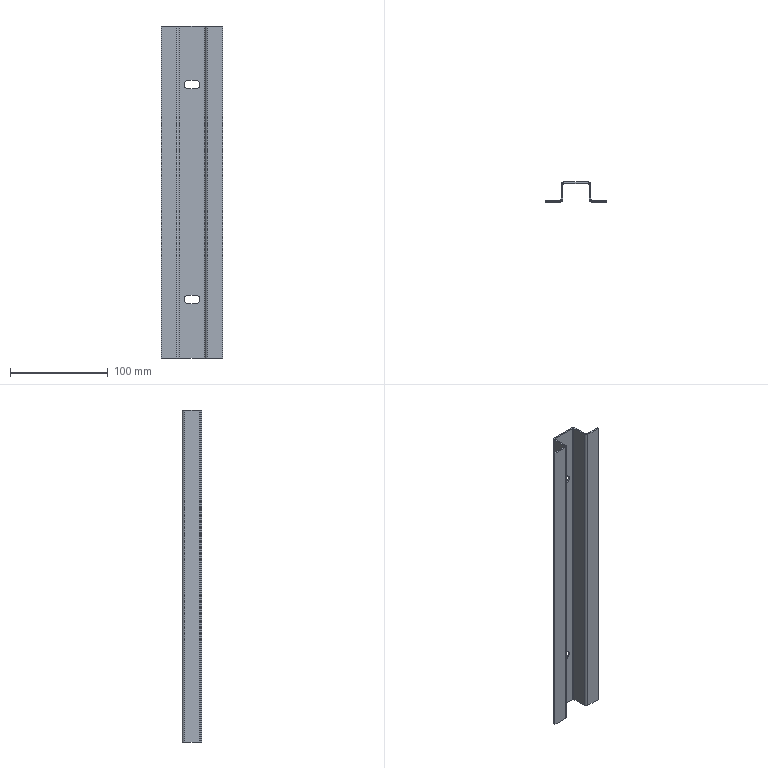Part | SolidWorks | features Cut 1, FlatPattern 1, LPattern 1, SMBaseFlange 1, SheetMetal 1 | 1 solid | 46 faces | box 63 x 20 x 340 mm | volume 49088 mm3 | plane 34 | cylinder 12 | commonest cylinder face diameters 2 x4 5 x4 9 x4
STEP:
#1=CARTESIAN_POINT('',(16.5,1.,170.));
#2=VERTEX_POINT('',#1);
#3=CARTESIAN_POINT('',(18.,1.,170.));
#4=VERTEX_POINT('',#3);
#5=CARTESIAN_POINT('',(16.5,1.,170.));
#6=DIRECTION('',(1.,0.,0.));
#7=VECTOR('',#6,1000.);
#8=LINE('',#5,#7);
#9=EDGE_CURVE('',#2,#4,#8,.T.);
#10=ORIENTED_EDGE('',*,*,#9,.F.);
#11=CARTESIAN_POINT('',(15.5,0.,170.));
#12=VERTEX_POINT('',#11);
#13=CARTESIAN_POINT('',(15.5,1.,170.));
#14=DIRECTION('',(0.,0.,1.));
#15=DIRECTION('',(-1.,0.,0.));
#16=AXIS2_PLACEMENT_3D('',#13,#14,#15);
#17=CIRCLE('',#16,1.);
#18=EDGE_CURVE('',#12,#2,#17,.T.);
#19=ORIENTED_EDGE('',*,*,#18,.F.);
#20=CARTESIAN_POINT('',(15.5,-1.5,170.));
#21=VERTEX_POINT('',#20);
#22=CARTESIAN_POINT('',(15.5,-1.5,170.));
#23=DIRECTION('',(0.,1.,0.));
#24=VECTOR('',#23,1000.);
#25=LINE('',#22,#24);
#26=EDGE_CURVE('',#21,#12,#25,.T.);
#27=ORIENTED_EDGE('',*,*,#26,.F.);
#28=CARTESIAN_POINT('',(15.5,1.,170.));
#29=DIRECTION('',(0.,0.,1.));
#30=DIRECTION('',(1.,0.,0.));
#31=AXIS2_PLACEMENT_3D('',#28,#29,#30);
#32=CIRCLE('',#31,2.5);
#33=EDGE_CURVE('',#21,#4,#32,.T.);
#34=ORIENTED_EDGE('',*,*,#33,.T.);
#35=EDGE_LOOP('',(#10,#19,#27,#34));
#36=FACE_OUTER_BOUND('',#35,.T.);
#37=CARTESIAN_POINT('',(16.5,1.,170.));
#38=DIRECTION('',(0.,0.,1.));
#39=DIRECTION('',(1.,0.,0.));
#40=AXIS2_PLACEMENT_3D('',#37,#38,#39);
#41=PLANE('',#40);
#42=ADVANCED_FACE('',(#36),#41,.T.);
#43=CARTESIAN_POINT('',(16.5,16.,170.));
#44=VERTEX_POINT('',#43);
#45=CARTESIAN_POINT('',(16.5,18.5,170.));
#46=DIRECTION('',(0.,1.,0.));
#47=VECTOR('',#46,1000.);
#48=LINE('',#45,#47);
#49=EDGE_CURVE('',#2,#44,#48,.T.);
#50=ORIENTED_EDGE('',*,*,#49,.F.);
#51=ORIENTED_EDGE('',*,*,#9,.T.);
#52=CARTESIAN_POINT('',(18.,16.,170.));
#53=VERTEX_POINT('',#52);
#54=CARTESIAN_POINT('',(18.,18.5,170.));
#55=DIRECTION('',(0.,1.,0.));
#56=VECTOR('',#55,1000.);
#57=LINE('',#54,#56);
#58=EDGE_CURVE('',#4,#53,#57,.T.);
#59=ORIENTED_EDGE('',*,*,#58,.T.);
#60=CARTESIAN_POINT('',(18.,16.,170.));
#61=DIRECTION('',(-1.,0.,0.));
#62=VECTOR('',#61,1000.);
#63=LINE('',#60,#62);
#64=EDGE_CURVE('',#53,#44,#63,.T.);
#65=ORIENTED_EDGE('',*,*,#64,.T.);
#66=EDGE_LOOP('',(#50,#51,#59,#65));
#67=FACE_OUTER_BOUND('',#66,.T.);
#68=CARTESIAN_POINT('',(15.5,-1.5,170.));
#69=DIRECTION('',(0.,0.,1.));
#70=DIRECTION('',(1.,0.,0.));
#71=AXIS2_PLACEMENT_3D('',#68,#69,#70);
#72=PLANE('',#71);
#73=ADVANCED_FACE('',(#67),#72,.T.);
#74=CARTESIAN_POINT('',(15.5,0.,-170.));
#75=VERTEX_POINT('',#74);
#76=CARTESIAN_POINT('',(15.5,-1.5,-170.));
#77=VERTEX_POINT('',#76);
#78=CARTESIAN_POINT('',(15.5,0.,-170.));
#79=DIRECTION('',(0.,-1.,0.));
#80=VECTOR('',#79,1000.);
#81=LINE('',#78,#80);
#82=EDGE_CURVE('',#75,#77,#81,.T.);
#83=ORIENTED_EDGE('',*,*,#82,.F.);
#84=CARTESIAN_POINT('',(16.5,1.,-170.));
#85=VERTEX_POINT('',#84);
#86=CARTESIAN_POINT('',(15.5,1.,-170.));
#87=DIRECTION('',(0.,0.,1.));
#88=DIRECTION('',(-1.,0.,0.));
#89=AXIS2_PLACEMENT_3D('',#86,#87,#88);
#90=CIRCLE('',#89,1.);
#91=EDGE_CURVE('',#75,#85,#90,.T.);
#92=ORIENTED_EDGE('',*,*,#91,.T.);
#93=CARTESIAN_POINT('',(18.,1.,-170.));
#94=VERTEX_POINT('',#93);
#95=CARTESIAN_POINT('',(18.,1.,-170.));
#96=DIRECTION('',(-1.,0.,0.));
#97=VECTOR('',#96,1000.);
#98=LINE('',#95,#97);
#99=EDGE_CURVE('',#94,#85,#98,.T.);
#100=ORIENTED_EDGE('',*,*,#99,.F.);
#101=CARTESIAN_POINT('',(15.5,1.,-170.));
#102=DIRECTION('',(0.,0.,1.));
#103=DIRECTION('',(1.,0.,0.));
#104=AXIS2_PLACEMENT_3D('',#101,#102,#103);
#105=CIRCLE('',#104,2.5);
#106=EDGE_CURVE('',#77,#94,#105,.T.);
#107=ORIENTED_EDGE('',*,*,#106,.F.);
#108=EDGE_LOOP('',(#83,#92,#100,#107));
#109=FACE_OUTER_BOUND('',#108,.T.);
#110=CARTESIAN_POINT('',(15.5,0.,-170.));
#111=DIRECTION('',(0.,0.,-1.));
#112=DIRECTION('',(-1.,0.,0.));
#113=AXIS2_PLACEMENT_3D('',#110,#111,#112);
#114=PLANE('',#113);
#115=ADVANCED_FACE('',(#109),#114,.T.);
#116=CARTESIAN_POINT('',(0.,0.,-170.));
#117=VERTEX_POINT('',#116);
#118=CARTESIAN_POINT('',(0.,0.,-170.));
#119=DIRECTION('',(1.,0.,0.));
#120=VECTOR('',#119,1000.);
#121=LINE('',#118,#120);
#122=EDGE_CURVE('',#117,#75,#121,.T.);
#123=ORIENTED_EDGE('',*,*,#122,.T.);
#124=ORIENTED_EDGE('',*,*,#82,.T.);
#125=CARTESIAN_POINT('',(0.,-1.5,-170.));
#126=VERTEX_POINT('',#125);
#127=CARTESIAN_POINT('',(0.,-1.5,-170.));
#128=DIRECTION('',(1.,0.,0.));
#129=VECTOR('',#128,1000.);
#130=LINE('',#127,#129);
#131=EDGE_CURVE('',#126,#77,#130,.T.);
#132=ORIENTED_EDGE('',*,*,#131,.F.);
#133=CARTESIAN_POINT('',(0.,-1.5,-170.));
#134=DIRECTION('',(0.,1.,0.));
#135=VECTOR('',#134,1000.);
#136=LINE('',#133,#135);
#137=EDGE_CURVE('',#126,#117,#136,.T.);
#138=ORIENTED_EDGE('',*,*,#137,.T.);
#139=EDGE_LOOP('',(#123,#124,#132,#138));
#140=FACE_OUTER_BOUND('',#139,.T.);
#141=CARTESIAN_POINT('',(18.,1.,-170.));
#142=DIRECTION('',(0.,0.,-1.));
#143=DIRECTION('',(-1.,0.,0.));
#144=AXIS2_PLACEMENT_3D('',#141,#142,#143);
#145=PLANE('',#144);
#146=ADVANCED_FACE('',(#140),#145,.T.);
#147=CARTESIAN_POINT('',(19.,18.5,170.));
#148=VERTEX_POINT('',#147);
#149=CARTESIAN_POINT('',(19.,17.,170.));
#150=VERTEX_POINT('',#149);
#151=CARTESIAN_POINT('',(19.,18.5,170.));
#152=DIRECTION('',(0.,-1.,0.));
#153=VECTOR('',#152,1000.);
#154=LINE('',#151,#153);
#155=EDGE_CURVE('',#148,#150,#154,.T.);
#156=ORIENTED_EDGE('',*,*,#155,.F.);
#157=CARTESIAN_POINT('',(19.,16.,170.));
#158=DIRECTION('',(0.,0.,-1.));
#159=DIRECTION('',(1.,0.,0.));
#160=AXIS2_PLACEMENT_3D('',#157,#158,#159);
#161=CIRCLE('',#160,2.5);
#162=EDGE_CURVE('',#44,#148,#161,.T.);
#163=ORIENTED_EDGE('',*,*,#162,.F.);
#164=ORIENTED_EDGE('',*,*,#64,.F.);
#165=CARTESIAN_POINT('',(19.,16.,170.));
#166=DIRECTION('',(0.,0.,-1.));
#167=DIRECTION('',(1.,0.,0.));
#168=AXIS2_PLACEMENT_3D('',#165,#166,#167);
#169=CIRCLE('',#168,1.);
#170=EDGE_CURVE('',#53,#150,#169,.T.);
#171=ORIENTED_EDGE('',*,*,#170,.T.);
#172=EDGE_LOOP('',(#156,#163,#164,#171));
#173=FACE_OUTER_BOUND('',#172,.T.);
#174=CARTESIAN_POINT('',(19.,18.5,170.));
#175=DIRECTION('',(0.,0.,1.));
#176=DIRECTION('',(1.,0.,0.));
#177=AXIS2_PLACEMENT_3D('',#174,#175,#176);
#178=PLANE('',#177);
#179=ADVANCED_FACE('',(#173),#178,.T.);
#180=CARTESIAN_POINT('',(44.,18.5,170.));
#181=VERTEX_POINT('',#180);
#182=CARTESIAN_POINT('',(16.5,18.5,170.));
#183=DIRECTION('',(1.,0.,0.));
#184=VECTOR('',#183,1000.);
#185=LINE('',#182,#184);
#186=EDGE_CURVE('',#148,#181,#185,.T.);
#187=ORIENTED_EDGE('',*,*,#186,.F.);
#188=ORIENTED_EDGE('',*,*,#155,.T.);
#189=CARTESIAN_POINT('',(44.,17.,170.));
#190=VERTEX_POINT('',#189);
#191=CARTESIAN_POINT('',(16.5,17.,170.));
#192=DIRECTION('',(1.,0.,0.));
#193=VECTOR('',#192,1000.);
#194=LINE('',#191,#193);
#195=EDGE_CURVE('',#150,#190,#194,.T.);
#196=ORIENTED_EDGE('',*,*,#195,.T.);
#197=CARTESIAN_POINT('',(44.,17.,170.));
#198=DIRECTION('',(0.,1.,0.));
#199=VECTOR('',#198,1000.);
#200=LINE('',#197,#199);
#201=EDGE_CURVE('',#190,#181,#200,.T.);
#202=ORIENTED_EDGE('',*,*,#201,.T.);
#203=EDGE_LOOP('',(#187,#188,#196,#202));
#204=FACE_OUTER_BOUND('',#203,.T.);
#205=CARTESIAN_POINT('',(18.,16.,170.));
#206=DIRECTION('',(0.,0.,1.));
#207=DIRECTION('',(1.,0.,0.));
#208=AXIS2_PLACEMENT_3D('',#205,#206,#207);
#209=PLANE('',#208);
#210=ADVANCED_FACE('',(#204),#209,.T.);
#211=CARTESIAN_POINT('',(16.5,16.,-170.));
#212=VERTEX_POINT('',#211);
#213=CARTESIAN_POINT('',(18.,16.,-170.));
#214=VERTEX_POINT('',#213);
#215=CARTESIAN_POINT('',(16.5,16.,-170.));
#216=DIRECTION('',(1.,0.,0.));
#217=VECTOR('',#216,1000.);
#218=LINE('',#215,#217);
#219=EDGE_CURVE('',#212,#214,#218,.T.);
#220=ORIENTED_EDGE('',*,*,#219,.F.);
#221=CARTESIAN_POINT('',(19.,18.5,-170.));
#222=VERTEX_POINT('',#221);
#223=CARTESIAN_POINT('',(19.,16.,-170.));
#224=DIRECTION('',(0.,0.,-1.));
#225=DIRECTION('',(1.,0.,0.));
#226=AXIS2_PLACEMENT_3D('',#223,#224,#225);
#227=CIRCLE('',#226,2.5);
#228=EDGE_CURVE('',#212,#222,#227,.T.);
#229=ORIENTED_EDGE('',*,*,#228,.T.);
#230=CARTESIAN_POINT('',(19.,17.,-170.));
#231=VERTEX_POINT('',#230);
#232=CARTESIAN_POINT('',(19.,17.,-170.));
#233=DIRECTION('',(0.,1.,0.));
#234=VECTOR('',#233,1000.);
#235=LINE('',#232,#234);
#236=EDGE_CURVE('',#231,#222,#235,.T.);
#237=ORIENTED_EDGE('',*,*,#236,.F.);
#238=CARTESIAN_POINT('',(19.,16.,-170.));
#239=DIRECTION('',(0.,0.,-1.));
#240=DIRECTION('',(1.,0.,0.));
#241=AXIS2_PLACEMENT_3D('',#238,#239,#240);
#242=CIRCLE('',#241,1.);
#243=EDGE_CURVE('',#214,#231,#242,.T.);
#244=ORIENTED_EDGE('',*,*,#243,.F.);
#245=EDGE_LOOP('',(#220,#229,#237,#244));
#246=FACE_OUTER_BOUND('',#245,.T.);
#247=CARTESIAN_POINT('',(16.5,16.,-170.));
#248=DIRECTION('',(0.,0.,-1.));
#249=DIRECTION('',(-1.,0.,0.));
#250=AXIS2_PLACEMENT_3D('',#247,#248,#249);
#251=PLANE('',#250);
#252=ADVANCED_FACE('',(#246),#251,.T.);
#253=CARTESIAN_POINT('',(16.5,18.5,-170.));
#254=DIRECTION('',(0.,1.,0.));
#255=VECTOR('',#254,1000.);
#256=LINE('',#253,#255);
#257=EDGE_CURVE('',#85,#212,#256,.T.);
#258=ORIENTED_EDGE('',*,*,#257,.T.);
#259=ORIENTED_EDGE('',*,*,#219,.T.);
#260=CARTESIAN_POINT('',(18.,18.5,-170.));
#261=DIRECTION('',(0.,1.,0.));
#262=VECTOR('',#261,1000.);
#263=LINE('',#260,#262);
#264=EDGE_CURVE('',#94,#214,#263,.T.);
#265=ORIENTED_EDGE('',*,*,#264,.F.);
#266=ORIENTED_EDGE('',*,*,#99,.T.);
#267=EDGE_LOOP('',(#258,#259,#265,#266));
#268=FACE_OUTER_BOUND('',#267,.T.);
#269=CARTESIAN_POINT('',(19.,17.,-170.));
#270=DIRECTION('',(0.,0.,-1.));
#271=DIRECTION('',(-1.,0.,0.));
#272=AXIS2_PLACEMENT_3D('',#269,#270,#271);
#273=PLANE('',#272);
#274=ADVANCED_FACE('',(#268),#273,.T.);
#275=CARTESIAN_POINT('',(46.5,16.,170.));
#276=VERTEX_POINT('',#275);
#277=CARTESIAN_POINT('',(45.,16.,170.));
#278=VERTEX_POINT('',#277);
#279=CARTESIAN_POINT('',(46.5,16.,170.));
#280=DIRECTION('',(-1.,0.,0.));
#281=VECTOR('',#280,1000.);
#282=LINE('',#279,#281);
#283=EDGE_CURVE('',#276,#278,#282,.T.);
#284=ORIENTED_EDGE('',*,*,#283,.F.);
#285=CARTESIAN_POINT('',(44.,16.,170.));
#286=DIRECTION('',(0.,0.,-1.));
#287=DIRECTION('',(1.,0.,0.));
#288=AXIS2_PLACEMENT_3D('',#285,#286,#287);
#289=CIRCLE('',#288,2.5);
#290=EDGE_CURVE('',#181,#276,#289,.T.);
#291=ORIENTED_EDGE('',*,*,#290,.F.);
#292=ORIENTED_EDGE('',*,*,#201,.F.);
#293=CARTESIAN_POINT('',(44.,16.,170.));
#294=DIRECTION('',(0.,0.,-1.));
#295=DIRECTION('',(1.,0.,0.));
#296=AXIS2_PLACEMENT_3D('',#293,#294,#295);
#297=CIRCLE('',#296,1.);
#298=EDGE_CURVE('',#190,#278,#297,.T.);
#299=ORIENTED_EDGE('',*,*,#298,.T.);
#300=EDGE_LOOP('',(#284,#291,#292,#299));
#301=FACE_OUTER_BOUND('',#300,.T.);
#302=CARTESIAN_POINT('',(46.5,16.,170.));
#303=DIRECTION('',(0.,0.,1.));
#304=DIRECTION('',(1.,0.,0.));
#305=AXIS2_PLACEMENT_3D('',#302,#303,#304);
#306=PLANE('',#305);
#307=ADVANCED_FACE('',(#301),#306,.T.);
#308=CARTESIAN_POINT('',(46.5,1.,170.));
#309=VERTEX_POINT('',#308);
#310=CARTESIAN_POINT('',(46.5,18.5,170.));
#311=DIRECTION('',(0.,-1.,0.));
#312=VECTOR('',#311,1000.);
#313=LINE('',#310,#312);
#314=EDGE_CURVE('',#276,#309,#313,.T.);
#315=ORIENTED_EDGE('',*,*,#314,.F.);
#316=ORIENTED_EDGE('',*,*,#283,.T.);
#317=CARTESIAN_POINT('',(45.,1.,170.));
#318=VERTEX_POINT('',#317);
#319=CARTESIAN_POINT('',(45.,18.5,170.));
#320=DIRECTION('',(0.,-1.,0.));
#321=VECTOR('',#320,1000.);
#322=LINE('',#319,#321);
#323=EDGE_CURVE('',#278,#318,#322,.T.);
#324=ORIENTED_EDGE('',*,*,#323,.T.);
#325=CARTESIAN_POINT('',(45.,1.,170.));
#326=DIRECTION('',(1.,0.,0.));
#327=VECTOR('',#326,1000.);
#328=LINE('',#325,#327);
#329=EDGE_CURVE('',#318,#309,#328,.T.);
#330=ORIENTED_EDGE('',*,*,#329,.T.);
#331=EDGE_LOOP('',(#315,#316,#324,#330));
#332=FACE_OUTER_BOUND('',#331,.T.);
#333=CARTESIAN_POINT('',(44.,17.,170.));
#334=DIRECTION('',(0.,0.,1.));
#335=DIRECTION('',(1.,0.,0.));
#336=AXIS2_PLACEMENT_3D('',#333,#334,#335);
#337=PLANE('',#336);
#338=ADVANCED_FACE('',(#332),#337,.T.);
#339=CARTESIAN_POINT('',(44.,18.5,-170.));
#340=VERTEX_POINT('',#339);
#341=CARTESIAN_POINT('',(44.,17.,-170.));
#342=VERTEX_POINT('',#341);
#343=CARTESIAN_POINT('',(44.,18.5,-170.));
#344=DIRECTION('',(0.,-1.,0.));
#345=VECTOR('',#344,1000.);
#346=LINE('',#343,#345);
#347=EDGE_CURVE('',#340,#342,#346,.T.);
#348=ORIENTED_EDGE('',*,*,#347,.F.);
#349=CARTESIAN_POINT('',(46.5,16.,-170.));
#350=VERTEX_POINT('',#349);
#351=CARTESIAN_POINT('',(44.,16.,-170.));
#352=DIRECTION('',(0.,0.,-1.));
#353=DIRECTION('',(1.,0.,0.));
#354=AXIS2_PLACEMENT_3D('',#351,#352,#353);
#355=CIRCLE('',#354,2.5);
#356=EDGE_CURVE('',#340,#350,#355,.T.);
#357=ORIENTED_EDGE('',*,*,#356,.T.);
#358=CARTESIAN_POINT('',(45.,16.,-170.));
#359=VERTEX_POINT('',#358);
#360=CARTESIAN_POINT('',(45.,16.,-170.));
#361=DIRECTION('',(1.,0.,0.));
#362=VECTOR('',#361,1000.);
#363=LINE('',#360,#362);
#364=EDGE_CURVE('',#359,#350,#363,.T.);
#365=ORIENTED_EDGE('',*,*,#364,.F.);
#366=CARTESIAN_POINT('',(44.,16.,-170.));
#367=DIRECTION('',(0.,0.,-1.));
#368=DIRECTION('',(1.,0.,0.));
#369=AXIS2_PLACEMENT_3D('',#366,#367,#368);
#370=CIRCLE('',#369,1.);
#371=EDGE_CURVE('',#342,#359,#370,.T.);
#372=ORIENTED_EDGE('',*,*,#371,.F.);
#373=EDGE_LOOP('',(#348,#357,#365,#372));
#374=FACE_OUTER_BOUND('',#373,.T.);
#375=CARTESIAN_POINT('',(44.,18.5,-170.));
#376=DIRECTION('',(0.,0.,-1.));
#377=DIRECTION('',(-1.,0.,0.));
#378=AXIS2_PLACEMENT_3D('',#375,#376,#377);
#379=PLANE('',#378);
#380=ADVANCED_FACE('',(#374),#379,.T.);
#381=CARTESIAN_POINT('',(16.5,18.5,-170.));
#382=DIRECTION('',(1.,0.,0.));
#383=VECTOR('',#382,1000.);
#384=LINE('',#381,#383);
#385=EDGE_CURVE('',#222,#340,#384,.T.);
#386=ORIENTED_EDGE('',*,*,#385,.T.);
#387=ORIENTED_EDGE('',*,*,#347,.T.);
#388=CARTESIAN_POINT('',(16.5,17.,-170.));
#389=DIRECTION('',(1.,0.,0.));
#390=VECTOR('',#389,1000.);
#391=LINE('',#388,#390);
#392=EDGE_CURVE('',#231,#342,#391,.T.);
#393=ORIENTED_EDGE('',*,*,#392,.F.);
#394=ORIENTED_EDGE('',*,*,#236,.T.);
#395=EDGE_LOOP('',(#386,#387,#393,#394));
#396=FACE_OUTER_BOUND('',#395,.T.);
#397=CARTESIAN_POINT('',(45.,16.,-170.));
#398=DIRECTION('',(0.,0.,-1.));
#399=DIRECTION('',(-1.,0.,0.));
#400=AXIS2_PLACEMENT_3D('',#397,#398,#399);
#401=PLANE('',#400);
#402=ADVANCED_FACE('',(#396),#401,.T.);
#403=CARTESIAN_POINT('',(47.5,0.,170.));
#404=VERTEX_POINT('',#403);
#405=CARTESIAN_POINT('',(47.5,-1.5,170.));
#406=VERTEX_POINT('',#405);
#407=CARTESIAN_POINT('',(47.5,0.,170.));
#408=DIRECTION('',(0.,-1.,0.));
#409=VECTOR('',#408,1000.);
#410=LINE('',#407,#409);
#411=EDGE_CURVE('',#404,#406,#410,.T.);
#412=ORIENTED_EDGE('',*,*,#411,.F.);
#413=CARTESIAN_POINT('',(47.5,1.,170.));
#414=DIRECTION('',(0.,0.,1.));
#415=DIRECTION('',(-1.,0.,0.));
#416=AXIS2_PLACEMENT_3D('',#413,#414,#415);
#417=CIRCLE('',#416,1.);
#418=EDGE_CURVE('',#309,#404,#417,.T.);
#419=ORIENTED_EDGE('',*,*,#418,.F.);
#420=ORIENTED_EDGE('',*,*,#329,.F.);
#421=CARTESIAN_POINT('',(47.5,1.,170.));
#422=DIRECTION('',(0.,0.,1.));
#423=DIRECTION('',(1.,0.,0.));
#424=AXIS2_PLACEMENT_3D('',#421,#422,#423);
#425=CIRCLE('',#424,2.5);
#426=EDGE_CURVE('',#318,#406,#425,.T.);
#427=ORIENTED_EDGE('',*,*,#426,.T.);
#428=EDGE_LOOP('',(#412,#419,#420,#427));
#429=FACE_OUTER_BOUND('',#428,.T.);
#430=CARTESIAN_POINT('',(47.5,0.,170.));
#431=DIRECTION('',(0.,0.,1.));
#432=DIRECTION('',(1.,0.,0.));
#433=AXIS2_PLACEMENT_3D('',#430,#431,#432);
#434=PLANE('',#433);
#435=ADVANCED_FACE('',(#429),#434,.T.);
#436=CARTESIAN_POINT('',(63.,0.,170.));
#437=VERTEX_POINT('',#436);
#438=CARTESIAN_POINT('',(46.5,0.,170.));
#439=DIRECTION('',(1.,0.,0.));
#440=VECTOR('',#439,1000.);
#441=LINE('',#438,#440);
#442=EDGE_CURVE('',#404,#437,#441,.T.);
#443=ORIENTED_EDGE('',*,*,#442,.F.);
#444=ORIENTED_EDGE('',*,*,#411,.T.);
#445=CARTESIAN_POINT('',(63.,-1.5,170.));
#446=VERTEX_POINT('',#445);
#447=CARTESIAN_POINT('',(46.5,-1.5,170.));
#448=DIRECTION('',(1.,0.,0.));
#449=VECTOR('',#448,1000.);
#450=LINE('',#447,#449);
#451=EDGE_CURVE('',#406,#446,#450,.T.);
#452=ORIENTED_EDGE('',*,*,#451,.T.);
#453=CARTESIAN_POINT('',(63.,0.,170.));
#454=DIRECTION('',(0.,-1.,0.));
#455=VECTOR('',#454,1000.);
#456=LINE('',#453,#455);
#457=EDGE_CURVE('',#437,#446,#456,.T.);
#458=ORIENTED_EDGE('',*,*,#457,.F.);
#459=EDGE_LOOP('',(#443,#444,#452,#458));
#460=FACE_OUTER_BOUND('',#459,.T.);
#461=CARTESIAN_POINT('',(45.,1.,170.));
#462=DIRECTION('',(0.,0.,1.));
#463=DIRECTION('',(1.,0.,0.));
#464=AXIS2_PLACEMENT_3D('',#461,#462,#463);
#465=PLANE('',#464);
#466=ADVANCED_FACE('',(#460),#465,.T.);
#467=CARTESIAN_POINT('',(46.5,1.,-170.));
#468=VERTEX_POINT('',#467);
#469=CARTESIAN_POINT('',(45.,1.,-170.));
#470=VERTEX_POINT('',#469);
#471=CARTESIAN_POINT('',(46.5,1.,-170.));
#472=DIRECTION('',(-1.,0.,0.));
#473=VECTOR('',#472,1000.);
#474=LINE('',#471,#473);
#475=EDGE_CURVE('',#468,#470,#474,.T.);
#476=ORIENTED_EDGE('',*,*,#475,.F.);
#477=CARTESIAN_POINT('',(47.5,0.,-170.));
#478=VERTEX_POINT('',#477);
#479=CARTESIAN_POINT('',(47.5,1.,-170.));
#480=DIRECTION('',(0.,0.,1.));
#481=DIRECTION('',(-1.,0.,0.));
#482=AXIS2_PLACEMENT_3D('',#479,#480,#481);
#483=CIRCLE('',#482,1.);
#484=EDGE_CURVE('',#468,#478,#483,.T.);
#485=ORIENTED_EDGE('',*,*,#484,.T.);
#486=CARTESIAN_POINT('',(47.5,-1.5,-170.));
#487=VERTEX_POINT('',#486);
#488=CARTESIAN_POINT('',(47.5,-1.5,-170.));
#489=DIRECTION('',(0.,1.,0.));
#490=VECTOR('',#489,1000.);
#491=LINE('',#488,#490);
#492=EDGE_CURVE('',#487,#478,#491,.T.);
#493=ORIENTED_EDGE('',*,*,#492,.F.);
#494=CARTESIAN_POINT('',(47.5,1.,-170.));
#495=DIRECTION('',(0.,0.,1.));
#496=DIRECTION('',(1.,0.,0.));
#497=AXIS2_PLACEMENT_3D('',#494,#495,#496);
#498=CIRCLE('',#497,2.5);
#499=EDGE_CURVE('',#470,#487,#498,.T.);
#500=ORIENTED_EDGE('',*,*,#499,.F.);
#501=EDGE_LOOP('',(#476,#485,#493,#500));
#502=FACE_OUTER_BOUND('',#501,.T.);
#503=CARTESIAN_POINT('',(46.5,1.,-170.));
#504=DIRECTION('',(0.,0.,-1.));
#505=DIRECTION('',(-1.,0.,0.));
#506=AXIS2_PLACEMENT_3D('',#503,#504,#505);
#507=PLANE('',#506);
#508=ADVANCED_FACE('',(#502),#507,.T.);
#509=CARTESIAN_POINT('',(46.5,18.5,-170.));
#510=DIRECTION('',(0.,-1.,0.));
#511=VECTOR('',#510,1000.);
#512=LINE('',#509,#511);
#513=EDGE_CURVE('',#350,#468,#512,.T.);
#514=ORIENTED_EDGE('',*,*,#513,.T.);
#515=ORIENTED_EDGE('',*,*,#475,.T.);
#516=CARTESIAN_POINT('',(45.,18.5,-170.));
#517=DIRECTION('',(0.,-1.,0.));
#518=VECTOR('',#517,1000.);
#519=LINE('',#516,#518);
#520=EDGE_CURVE('',#359,#470,#519,.T.);
#521=ORIENTED_EDGE('',*,*,#520,.F.);
#522=ORIENTED_EDGE('',*,*,#364,.T.);
#523=EDGE_LOOP('',(#514,#515,#521,#522));
#524=FACE_OUTER_BOUND('',#523,.T.);
#525=CARTESIAN_POINT('',(47.5,-1.5,-170.));
#526=DIRECTION('',(0.,0.,-1.));
#527=DIRECTION('',(-1.,0.,0.));
#528=AXIS2_PLACEMENT_3D('',#525,#526,#527);
#529=PLANE('',#528);
#530=ADVANCED_FACE('',(#524),#529,.T.);
#531=CARTESIAN_POINT('',(63.,-1.5,-170.));
#532=VERTEX_POINT('',#531);
#533=CARTESIAN_POINT('',(46.5,-1.5,-170.));
#534=DIRECTION('',(1.,0.,0.));
#535=VECTOR('',#534,1000.);
#536=LINE('',#533,#535);
#537=EDGE_CURVE('',#487,#532,#536,.T.);
#538=ORIENTED_EDGE('',*,*,#537,.T.);
#539=CARTESIAN_POINT('',(63.,-1.5,170.));
#540=DIRECTION('',(0.,0.,-1.));
#541=VECTOR('',#540,1000.);
#542=LINE('',#539,#541);
#543=EDGE_CURVE('',#446,#532,#542,.T.);
#544=ORIENTED_EDGE('',*,*,#543,.F.);
#545=ORIENTED_EDGE('',*,*,#451,.F.);
#546=CARTESIAN_POINT('',(47.5,-1.5,170.));
#547=DIRECTION('',(0.,0.,-1.));
#548=VECTOR('',#547,1000.);
#549=LINE('',#546,#548);
#550=EDGE_CURVE('',#406,#487,#549,.T.);
#551=ORIENTED_EDGE('',*,*,#550,.T.);
#552=EDGE_LOOP('',(#538,#544,#545,#551));
#553=FACE_OUTER_BOUND('',#552,.T.);
#554=CARTESIAN_POINT('',(46.5,-1.5,170.));
#555=DIRECTION('',(0.,1.,0.));
#556=DIRECTION('',(0.,0.,1.));
#557=AXIS2_PLACEMENT_3D('',#554,#555,#556);
#558=PLANE('',#557);
#559=ADVANCED_FACE('',(#553),#558,.F.);
#560=CARTESIAN_POINT('',(63.,0.,-170.));
#561=VERTEX_POINT('',#560);
#562=CARTESIAN_POINT('',(63.,0.,-170.));
#563=DIRECTION('',(0.,-1.,0.));
#564=VECTOR('',#563,1000.);
#565=LINE('',#562,#564);
#566=EDGE_CURVE('',#561,#532,#565,.T.);
#567=ORIENTED_EDGE('',*,*,#566,.F.);
#568=CARTESIAN_POINT('',(63.,0.,170.));
#569=DIRECTION('',(0.,0.,-1.));
#570=VECTOR('',#569,1000.);
#571=LINE('',#568,#570);
#572=EDGE_CURVE('',#437,#561,#571,.T.);
#573=ORIENTED_EDGE('',*,*,#572,.F.);
#574=ORIENTED_EDGE('',*,*,#457,.T.);
#575=ORIENTED_EDGE('',*,*,#543,.T.);
#576=EDGE_LOOP('',(#567,#573,#574,#575));
#577=FACE_OUTER_BOUND('',#576,.T.);
#578=CARTESIAN_POINT('',(63.,0.,170.));
#579=DIRECTION('',(1.,0.,0.));
#580=DIRECTION('',(0.,0.,-1.));
#581=AXIS2_PLACEMENT_3D('',#578,#579,#580);
#582=PLANE('',#581);
#583=ADVANCED_FACE('',(#577),#582,.T.);
#584=CARTESIAN_POINT('',(46.5,0.,-170.));
#585=DIRECTION('',(1.,0.,0.));
#586=VECTOR('',#585,1000.);
#587=LINE('',#584,#586);
#588=EDGE_CURVE('',#478,#561,#587,.T.);
#589=ORIENTED_EDGE('',*,*,#588,.F.);
#590=CARTESIAN_POINT('',(47.5,0.,170.));
#591=DIRECTION('',(0.,0.,-1.));
#592=VECTOR('',#591,1000.);
#593=LINE('',#590,#592);
#594=EDGE_CURVE('',#404,#478,#593,.T.);
#595=ORIENTED_EDGE('',*,*,#594,.F.);
#596=ORIENTED_EDGE('',*,*,#442,.T.);
#597=ORIENTED_EDGE('',*,*,#572,.T.);
#598=EDGE_LOOP('',(#589,#595,#596,#597));
#599=FACE_OUTER_BOUND('',#598,.T.);
#600=CARTESIAN_POINT('',(46.5,0.,170.));
#601=DIRECTION('',(0.,1.,0.));
#602=DIRECTION('',(0.,0.,1.));
#603=AXIS2_PLACEMENT_3D('',#600,#601,#602);
#604=PLANE('',#603);
#605=ADVANCED_FACE('',(#599),#604,.T.);
#606=ORIENTED_EDGE('',*,*,#484,.F.);
#607=CARTESIAN_POINT('',(46.5,1.,170.));
#608=DIRECTION('',(0.,0.,-1.));
#609=VECTOR('',#608,1000.);
#610=LINE('',#607,#609);
#611=EDGE_CURVE('',#309,#468,#610,.T.);
#612=ORIENTED_EDGE('',*,*,#611,.F.);
#613=ORIENTED_EDGE('',*,*,#418,.T.);
#614=ORIENTED_EDGE('',*,*,#594,.T.);
#615=EDGE_LOOP('',(#606,#612,#613,#614));
#616=FACE_OUTER_BOUND('',#615,.T.);
#617=CARTESIAN_POINT('',(47.5,1.,170.));
#618=DIRECTION('',(0.,0.,-1.));
#619=DIRECTION('',(-1.,0.,0.));
#620=AXIS2_PLACEMENT_3D('',#617,#618,#619);
#621=CYLINDRICAL_SURFACE('',#620,1.);
#622=ADVANCED_FACE('',(#616),#621,.F.);
#623=ORIENTED_EDGE('',*,*,#513,.F.);
#624=CARTESIAN_POINT('',(46.5,16.,170.));
#625=DIRECTION('',(0.,0.,-1.));
#626=VECTOR('',#625,1000.);
#627=LINE('',#624,#626);
#628=EDGE_CURVE('',#276,#350,#627,.T.);
#629=ORIENTED_EDGE('',*,*,#628,.F.);
#630=ORIENTED_EDGE('',*,*,#314,.T.);
#631=ORIENTED_EDGE('',*,*,#611,.T.);
#632=EDGE_LOOP('',(#623,#629,#630,#631));
#633=FACE_OUTER_BOUND('',#632,.T.);
#634=CARTESIAN_POINT('',(46.5,18.5,170.));
#635=DIRECTION('',(1.,0.,0.));
#636=DIRECTION('',(0.,0.,-1.));
#637=AXIS2_PLACEMENT_3D('',#634,#635,#636);
#638=PLANE('',#637);
#639=ADVANCED_FACE('',(#633),#638,.T.);
#640=ORIENTED_EDGE('',*,*,#356,.F.);
#641=CARTESIAN_POINT('',(44.,18.5,170.));
#642=DIRECTION('',(0.,0.,-1.));
#643=VECTOR('',#642,1000.);
#644=LINE('',#641,#643);
#645=EDGE_CURVE('',#181,#340,#644,.T.);
#646=ORIENTED_EDGE('',*,*,#645,.F.);
#647=ORIENTED_EDGE('',*,*,#290,.T.);
#648=ORIENTED_EDGE('',*,*,#628,.T.);
#649=EDGE_LOOP('',(#640,#646,#647,#648));
#650=FACE_OUTER_BOUND('',#649,.T.);
#651=CARTESIAN_POINT('',(44.,16.,170.));
#652=DIRECTION('',(0.,0.,-1.));
#653=DIRECTION('',(-1.,0.,0.));
#654=AXIS2_PLACEMENT_3D('',#651,#652,#653);
#655=CYLINDRICAL_SURFACE('',#654,2.5);
#656=ADVANCED_FACE('',(#650),#655,.T.);
#657=CARTESIAN_POINT('',(35.,18.5,-105.5));
#658=VERTEX_POINT('',#657);
#659=CARTESIAN_POINT('',(35.,18.5,-114.5));
#660=VERTEX_POINT('',#659);
#661=CARTESIAN_POINT('',(35.,18.5,-110.));
#662=DIRECTION('',(0.,1.,0.));
#663=DIRECTION('',(0.,0.,1.));
#664=AXIS2_PLACEMENT_3D('',#661,#662,#663);
#665=CIRCLE('',#664,4.5);
#666=EDGE_CURVE('',#658,#660,#665,.T.);
#667=ORIENTED_EDGE('',*,*,#666,.F.);
#668=CARTESIAN_POINT('',(28.,18.5,-105.5));
#669=VERTEX_POINT('',#668);
#670=CARTESIAN_POINT('',(35.,18.5,-105.5));
#671=DIRECTION('',(1.,0.,0.));
#672=VECTOR('',#671,1000.);
#673=LINE('',#670,#672);
#674=EDGE_CURVE('',#669,#658,#673,.T.);
#675=ORIENTED_EDGE('',*,*,#674,.F.);
#676=CARTESIAN_POINT('',(28.,18.5,-114.5));
#677=VERTEX_POINT('',#676);
#678=CARTESIAN_POINT('',(28.,18.5,-110.));
#679=DIRECTION('',(0.,1.,0.));
#680=DIRECTION('',(0.,0.,1.));
#681=AXIS2_PLACEMENT_3D('',#678,#679,#680);
#682=CIRCLE('',#681,4.5);
#683=EDGE_CURVE('',#677,#669,#682,.T.);
#684=ORIENTED_EDGE('',*,*,#683,.F.);
#685=CARTESIAN_POINT('',(35.,18.5,-114.5));
#686=DIRECTION('',(-1.,0.,0.));
#687=VECTOR('',#686,1000.);
#688=LINE('',#685,#687);
#689=EDGE_CURVE('',#660,#677,#688,.T.);
#690=ORIENTED_EDGE('',*,*,#689,.F.);
#691=EDGE_LOOP('',(#667,#675,#684,#690));
#692=FACE_BOUND('',#691,.T.);
#693=CARTESIAN_POINT('',(35.,18.5,114.5));
#694=VERTEX_POINT('',#693);
#695=CARTESIAN_POINT('',(35.,18.5,105.5));
#696=VERTEX_POINT('',#695);
#697=CARTESIAN_POINT('',(35.,18.5,110.));
#698=DIRECTION('',(0.,1.,0.));
#699=DIRECTION('',(0.,0.,1.));
#700=AXIS2_PLACEMENT_3D('',#697,#698,#699);
#701=CIRCLE('',#700,4.5);
#702=EDGE_CURVE('',#694,#696,#701,.T.);
#703=ORIENTED_EDGE('',*,*,#702,.F.);
#704=CARTESIAN_POINT('',(28.,18.5,114.5));
#705=VERTEX_POINT('',#704);
#706=CARTESIAN_POINT('',(35.,18.5,114.5));
#707=DIRECTION('',(1.,0.,0.));
#708=VECTOR('',#707,1000.);
#709=LINE('',#706,#708);
#710=EDGE_CURVE('',#705,#694,#709,.T.);
#711=ORIENTED_EDGE('',*,*,#710,.F.);
#712=CARTESIAN_POINT('',(28.,18.5,105.5));
#713=VERTEX_POINT('',#712);
#714=CARTESIAN_POINT('',(28.,18.5,110.));
#715=DIRECTION('',(0.,1.,0.));
#716=DIRECTION('',(0.,0.,1.));
#717=AXIS2_PLACEMENT_3D('',#714,#715,#716);
#718=CIRCLE('',#717,4.5);
#719=EDGE_CURVE('',#713,#705,#718,.T.);
#720=ORIENTED_EDGE('',*,*,#719,.F.);
#721=CARTESIAN_POINT('',(35.,18.5,105.5));
#722=DIRECTION('',(-1.,0.,0.));
#723=VECTOR('',#722,1000.);
#724=LINE('',#721,#723);
#725=EDGE_CURVE('',#696,#713,#724,.T.);
#726=ORIENTED_EDGE('',*,*,#725,.F.);
#727=EDGE_LOOP('',(#703,#711,#720,#726));
#728=FACE_BOUND('',#727,.T.);
#729=ORIENTED_EDGE('',*,*,#385,.F.);
#730=CARTESIAN_POINT('',(19.,18.5,170.));
#731=DIRECTION('',(0.,0.,-1.));
#732=VECTOR('',#731,1000.);
#733=LINE('',#730,#732);
#734=EDGE_CURVE('',#148,#222,#733,.T.);
#735=ORIENTED_EDGE('',*,*,#734,.F.);
#736=ORIENTED_EDGE('',*,*,#186,.T.);
#737=ORIENTED_EDGE('',*,*,#645,.T.);
#738=EDGE_LOOP('',(#729,#735,#736,#737));
#739=FACE_OUTER_BOUND('',#738,.T.);
#740=CARTESIAN_POINT('',(16.5,18.5,170.));
#741=DIRECTION('',(0.,1.,0.));
#742=DIRECTION('',(0.,0.,1.));
#743=AXIS2_PLACEMENT_3D('',#740,#741,#742);
#744=PLANE('',#743);
#745=ADVANCED_FACE('',(#692,#728,#739),#744,.T.);
#746=ORIENTED_EDGE('',*,*,#228,.F.);
#747=CARTESIAN_POINT('',(16.5,16.,170.));
#748=DIRECTION('',(0.,0.,-1.));
#749=VECTOR('',#748,1000.);
#750=LINE('',#747,#749);
#751=EDGE_CURVE('',#44,#212,#750,.T.);
#752=ORIENTED_EDGE('',*,*,#751,.F.);
#753=ORIENTED_EDGE('',*,*,#162,.T.);
#754=ORIENTED_EDGE('',*,*,#734,.T.);
#755=EDGE_LOOP('',(#746,#752,#753,#754));
#756=FACE_OUTER_BOUND('',#755,.T.);
#757=CARTESIAN_POINT('',(19.,16.,170.));
#758=DIRECTION('',(0.,0.,-1.));
#759=DIRECTION('',(-1.,0.,0.));
#760=AXIS2_PLACEMENT_3D('',#757,#758,#759);
#761=CYLINDRICAL_SURFACE('',#760,2.5);
#762=ADVANCED_FACE('',(#756),#761,.T.);
#763=ORIENTED_EDGE('',*,*,#257,.F.);
#764=CARTESIAN_POINT('',(16.5,1.,170.));
#765=DIRECTION('',(0.,0.,-1.));
#766=VECTOR('',#765,1000.);
#767=LINE('',#764,#766);
#768=EDGE_CURVE('',#2,#85,#767,.T.);
#769=ORIENTED_EDGE('',*,*,#768,.F.);
#770=ORIENTED_EDGE('',*,*,#49,.T.);
#771=ORIENTED_EDGE('',*,*,#751,.T.);
#772=EDGE_LOOP('',(#763,#769,#770,#771));
#773=FACE_OUTER_BOUND('',#772,.T.);
#774=CARTESIAN_POINT('',(16.5,18.5,170.));
#775=DIRECTION('',(-1.,0.,0.));
#776=DIRECTION('',(0.,0.,1.));
#777=AXIS2_PLACEMENT_3D('',#774,#775,#776);
#778=PLANE('',#777);
#779=ADVANCED_FACE('',(#773),#778,.T.);
#780=ORIENTED_EDGE('',*,*,#91,.F.);
#781=CARTESIAN_POINT('',(15.5,0.,170.));
#782=DIRECTION('',(0.,0.,-1.));
#783=VECTOR('',#782,1000.);
#784=LINE('',#781,#783);
#785=EDGE_CURVE('',#12,#75,#784,.T.);
#786=ORIENTED_EDGE('',*,*,#785,.F.);
#787=ORIENTED_EDGE('',*,*,#18,.T.);
#788=ORIENTED_EDGE('',*,*,#768,.T.);
#789=EDGE_LOOP('',(#780,#786,#787,#788));
#790=FACE_OUTER_BOUND('',#789,.T.);
#791=CARTESIAN_POINT('',(15.5,1.,170.));
#792=DIRECTION('',(0.,0.,-1.));
#793=DIRECTION('',(-1.,0.,0.));
#794=AXIS2_PLACEMENT_3D('',#791,#792,#793);
#795=CYLINDRICAL_SURFACE('',#794,1.);
#796=ADVANCED_FACE('',(#790),#795,.F.);
#797=ORIENTED_EDGE('',*,*,#122,.F.);
#798=CARTESIAN_POINT('',(0.,0.,170.));
#799=VERTEX_POINT('',#798);
#800=CARTESIAN_POINT('',(0.,0.,170.));
#801=DIRECTION('',(0.,0.,-1.));
#802=VECTOR('',#801,1000.);
#803=LINE('',#800,#802);
#804=EDGE_CURVE('',#799,#117,#803,.T.);
#805=ORIENTED_EDGE('',*,*,#804,.F.);
#806=CARTESIAN_POINT('',(0.,0.,170.));
#807=DIRECTION('',(1.,0.,0.));
#808=VECTOR('',#807,1000.);
#809=LINE('',#806,#808);
#810=EDGE_CURVE('',#799,#12,#809,.T.);
#811=ORIENTED_EDGE('',*,*,#810,.T.);
#812=ORIENTED_EDGE('',*,*,#785,.T.);
#813=EDGE_LOOP('',(#797,#805,#811,#812));
#814=FACE_OUTER_BOUND('',#813,.T.);
#815=CARTESIAN_POINT('',(0.,0.,170.));
#816=DIRECTION('',(0.,1.,0.));
#817=DIRECTION('',(0.,0.,1.));
#818=AXIS2_PLACEMENT_3D('',#815,#816,#817);
#819=PLANE('',#818);
#820=ADVANCED_FACE('',(#814),#819,.T.);
#821=ORIENTED_EDGE('',*,*,#137,.F.);
#822=CARTESIAN_POINT('',(0.,-1.5,170.));
#823=VERTEX_POINT('',#822);
#824=CARTESIAN_POINT('',(0.,-1.5,170.));
#825=DIRECTION('',(0.,0.,-1.));
#826=VECTOR('',#825,1000.);
#827=LINE('',#824,#826);
#828=EDGE_CURVE('',#823,#126,#827,.T.);
#829=ORIENTED_EDGE('',*,*,#828,.F.);
#830=CARTESIAN_POINT('',(0.,-1.5,170.));
#831=DIRECTION('',(0.,1.,0.));
#832=VECTOR('',#831,1000.);
#833=LINE('',#830,#832);
#834=EDGE_CURVE('',#823,#799,#833,.T.);
#835=ORIENTED_EDGE('',*,*,#834,.T.);
#836=ORIENTED_EDGE('',*,*,#804,.T.);
#837=EDGE_LOOP('',(#821,#829,#835,#836));
#838=FACE_OUTER_BOUND('',#837,.T.);
#839=CARTESIAN_POINT('',(0.,-1.5,170.));
#840=DIRECTION('',(-1.,0.,0.));
#841=DIRECTION('',(0.,0.,1.));
#842=AXIS2_PLACEMENT_3D('',#839,#840,#841);
#843=PLANE('',#842);
#844=ADVANCED_FACE('',(#838),#843,.T.);
#845=ORIENTED_EDGE('',*,*,#131,.T.);
#846=CARTESIAN_POINT('',(15.5,-1.5,170.));
#847=DIRECTION('',(0.,0.,-1.));
#848=VECTOR('',#847,1000.);
#849=LINE('',#846,#848);
#850=EDGE_CURVE('',#21,#77,#849,.T.);
#851=ORIENTED_EDGE('',*,*,#850,.F.);
#852=CARTESIAN_POINT('',(0.,-1.5,170.));
#853=DIRECTION('',(1.,0.,0.));
#854=VECTOR('',#853,1000.);
#855=LINE('',#852,#854);
#856=EDGE_CURVE('',#823,#21,#855,.T.);
#857=ORIENTED_EDGE('',*,*,#856,.F.);
#858=ORIENTED_EDGE('',*,*,#828,.T.);
#859=EDGE_LOOP('',(#845,#851,#857,#858));
#860=FACE_OUTER_BOUND('',#859,.T.);
#861=CARTESIAN_POINT('',(0.,-1.5,170.));
#862=DIRECTION('',(0.,1.,0.));
#863=DIRECTION('',(0.,0.,1.));
#864=AXIS2_PLACEMENT_3D('',#861,#862,#863);
#865=PLANE('',#864);
#866=ADVANCED_FACE('',(#860),#865,.F.);
#867=ORIENTED_EDGE('',*,*,#106,.T.);
#868=CARTESIAN_POINT('',(18.,1.,170.));
#869=DIRECTION('',(0.,0.,-1.));
#870=VECTOR('',#869,1000.);
#871=LINE('',#868,#870);
#872=EDGE_CURVE('',#4,#94,#871,.T.);
#873=ORIENTED_EDGE('',*,*,#872,.F.);
#874=ORIENTED_EDGE('',*,*,#33,.F.);
#875=ORIENTED_EDGE('',*,*,#850,.T.);
#876=EDGE_LOOP('',(#867,#873,#874,#875));
#877=FACE_OUTER_BOUND('',#876,.T.);
#878=CARTESIAN_POINT('',(15.5,1.,170.));
#879=DIRECTION('',(0.,0.,-1.));
#880=DIRECTION('',(-1.,0.,0.));
#881=AXIS2_PLACEMENT_3D('',#878,#879,#880);
#882=CYLINDRICAL_SURFACE('',#881,2.5);
#883=ADVANCED_FACE('',(#877),#882,.T.);
#884=ORIENTED_EDGE('',*,*,#264,.T.);
#885=CARTESIAN_POINT('',(18.,16.,170.));
#886=DIRECTION('',(0.,0.,-1.));
#887=VECTOR('',#886,1000.);
#888=LINE('',#885,#887);
#889=EDGE_CURVE('',#53,#214,#888,.T.);
#890=ORIENTED_EDGE('',*,*,#889,.F.);
#891=ORIENTED_EDGE('',*,*,#58,.F.);
#892=ORIENTED_EDGE('',*,*,#872,.T.);
#893=EDGE_LOOP('',(#884,#890,#891,#892));
#894=FACE_OUTER_BOUND('',#893,.T.);
#895=CARTESIAN_POINT('',(18.,18.5,170.));
#896=DIRECTION('',(-1.,0.,0.));
#897=DIRECTION('',(0.,0.,1.));
#898=AXIS2_PLACEMENT_3D('',#895,#896,#897);
#899=PLANE('',#898);
#900=ADVANCED_FACE('',(#894),#899,.F.);
#901=ORIENTED_EDGE('',*,*,#243,.T.);
#902=CARTESIAN_POINT('',(19.,17.,170.));
#903=DIRECTION('',(0.,0.,-1.));
#904=VECTOR('',#903,1000.);
#905=LINE('',#902,#904);
#906=EDGE_CURVE('',#150,#231,#905,.T.);
#907=ORIENTED_EDGE('',*,*,#906,.F.);
#908=ORIENTED_EDGE('',*,*,#170,.F.);
#909=ORIENTED_EDGE('',*,*,#889,.T.);
#910=EDGE_LOOP('',(#901,#907,#908,#909));
#911=FACE_OUTER_BOUND('',#910,.T.);
#912=CARTESIAN_POINT('',(19.,16.,170.));
#913=DIRECTION('',(0.,0.,-1.));
#914=DIRECTION('',(-1.,0.,0.));
#915=AXIS2_PLACEMENT_3D('',#912,#913,#914);
#916=CYLINDRICAL_SURFACE('',#915,1.);
#917=ADVANCED_FACE('',(#911),#916,.F.);
#918=CARTESIAN_POINT('',(28.,17.,-105.5));
#919=VERTEX_POINT('',#918);
#920=CARTESIAN_POINT('',(35.,17.,-105.5));
#921=VERTEX_POINT('',#920);
#922=CARTESIAN_POINT('',(35.,17.,-105.5));
#923=DIRECTION('',(1.,0.,0.));
#924=VECTOR('',#923,1000.);
#925=LINE('',#922,#924);
#926=EDGE_CURVE('',#919,#921,#925,.T.);
#927=ORIENTED_EDGE('',*,*,#926,.T.);
#928=CARTESIAN_POINT('',(35.,17.,-114.5));
#929=VERTEX_POINT('',#928);
#930=CARTESIAN_POINT('',(35.,17.,-110.));
#931=DIRECTION('',(0.,1.,0.));
#932=DIRECTION('',(0.,0.,1.));
#933=AXIS2_PLACEMENT_3D('',#930,#931,#932);
#934=CIRCLE('',#933,4.5);
#935=EDGE_CURVE('',#921,#929,#934,.T.);
#936=ORIENTED_EDGE('',*,*,#935,.T.);
#937=CARTESIAN_POINT('',(28.,17.,-114.5));
#938=VERTEX_POINT('',#937);
#939=CARTESIAN_POINT('',(35.,17.,-114.5));
#940=DIRECTION('',(-1.,0.,0.));
#941=VECTOR('',#940,1000.);
#942=LINE('',#939,#941);
#943=EDGE_CURVE('',#929,#938,#942,.T.);
#944=ORIENTED_EDGE('',*,*,#943,.T.);
#945=CARTESIAN_POINT('',(28.,17.,-110.));
#946=DIRECTION('',(0.,1.,0.));
#947=DIRECTION('',(0.,0.,1.));
#948=AXIS2_PLACEMENT_3D('',#945,#946,#947);
#949=CIRCLE('',#948,4.5);
#950=EDGE_CURVE('',#938,#919,#949,.T.);
#951=ORIENTED_EDGE('',*,*,#950,.T.);
#952=EDGE_LOOP('',(#927,#936,#944,#951));
#953=FACE_BOUND('',#952,.T.);
#954=CARTESIAN_POINT('',(28.,17.,114.5));
#955=VERTEX_POINT('',#954);
#956=CARTESIAN_POINT('',(35.,17.,114.5));
#957=VERTEX_POINT('',#956);
#958=CARTESIAN_POINT('',(35.,17.,114.5));
#959=DIRECTION('',(1.,0.,0.));
#960=VECTOR('',#959,1000.);
#961=LINE('',#958,#960);
#962=EDGE_CURVE('',#955,#957,#961,.T.);
#963=ORIENTED_EDGE('',*,*,#962,.T.);
#964=CARTESIAN_POINT('',(35.,17.,105.5));
#965=VERTEX_POINT('',#964);
#966=CARTESIAN_POINT('',(35.,17.,110.));
#967=DIRECTION('',(0.,1.,0.));
#968=DIRECTION('',(0.,0.,1.));
#969=AXIS2_PLACEMENT_3D('',#966,#967,#968);
#970=CIRCLE('',#969,4.5);
#971=EDGE_CURVE('',#957,#965,#970,.T.);
#972=ORIENTED_EDGE('',*,*,#971,.T.);
#973=CARTESIAN_POINT('',(28.,17.,105.5));
#974=VERTEX_POINT('',#973);
#975=CARTESIAN_POINT('',(35.,17.,105.5));
#976=DIRECTION('',(-1.,0.,0.));
#977=VECTOR('',#976,1000.);
#978=LINE('',#975,#977);
#979=EDGE_CURVE('',#965,#974,#978,.T.);
#980=ORIENTED_EDGE('',*,*,#979,.T.);
#981=CARTESIAN_POINT('',(28.,17.,110.));
#982=DIRECTION('',(0.,1.,0.));
#983=DIRECTION('',(0.,0.,1.));
#984=AXIS2_PLACEMENT_3D('',#981,#982,#983);
#985=CIRCLE('',#984,4.5);
#986=EDGE_CURVE('',#974,#955,#985,.T.);
#987=ORIENTED_EDGE('',*,*,#986,.T.);
#988=EDGE_LOOP('',(#963,#972,#980,#987));
#989=FACE_BOUND('',#988,.T.);
#990=ORIENTED_EDGE('',*,*,#392,.T.);
#991=CARTESIAN_POINT('',(44.,17.,170.));
#992=DIRECTION('',(0.,0.,-1.));
#993=VECTOR('',#992,1000.);
#994=LINE('',#991,#993);
#995=EDGE_CURVE('',#190,#342,#994,.T.);
#996=ORIENTED_EDGE('',*,*,#995,.F.);
#997=ORIENTED_EDGE('',*,*,#195,.F.);
#998=ORIENTED_EDGE('',*,*,#906,.T.);
#999=EDGE_LOOP('',(#990,#996,#997,#998));
#1000=FACE_OUTER_BOUND('',#999,.T.);
#1001=CARTESIAN_POINT('',(16.5,17.,170.));
#1002=DIRECTION('',(0.,1.,0.));
#1003=DIRECTION('',(0.,0.,1.));
#1004=AXIS2_PLACEMENT_3D('',#1001,#1002,#1003);
#1005=PLANE('',#1004);
#1006=ADVANCED_FACE('',(#953,#989,#1000),#1005,.F.);
#1007=ORIENTED_EDGE('',*,*,#371,.T.);
#1008=CARTESIAN_POINT('',(45.,16.,170.));
#1009=DIRECTION('',(0.,0.,-1.));
#1010=VECTOR('',#1009,1000.);
#1011=LINE('',#1008,#1010);
#1012=EDGE_CURVE('',#278,#359,#1011,.T.);
#1013=ORIENTED_EDGE('',*,*,#1012,.F.);
#1014=ORIENTED_EDGE('',*,*,#298,.F.);
#1015=ORIENTED_EDGE('',*,*,#995,.T.);
#1016=EDGE_LOOP('',(#1007,#1013,#1014,#1015));
#1017=FACE_OUTER_BOUND('',#1016,.T.);
#1018=CARTESIAN_POINT('',(44.,16.,170.));
#1019=DIRECTION('',(0.,0.,-1.));
#1020=DIRECTION('',(-1.,0.,0.));
#1021=AXIS2_PLACEMENT_3D('',#1018,#1019,#1020);
#1022=CYLINDRICAL_SURFACE('',#1021,1.);
#1023=ADVANCED_FACE('',(#1017),#1022,.F.);
#1024=ORIENTED_EDGE('',*,*,#520,.T.);
#1025=CARTESIAN_POINT('',(45.,1.,170.));
#1026=DIRECTION('',(0.,0.,-1.));
#1027=VECTOR('',#1026,1000.);
#1028=LINE('',#1025,#1027);
#1029=EDGE_CURVE('',#318,#470,#1028,.T.);
#1030=ORIENTED_EDGE('',*,*,#1029,.F.);
#1031=ORIENTED_EDGE('',*,*,#323,.F.);
#1032=ORIENTED_EDGE('',*,*,#1012,.T.);
#1033=EDGE_LOOP('',(#1024,#1030,#1031,#1032));
#1034=FACE_OUTER_BOUND('',#1033,.T.);
#1035=CARTESIAN_POINT('',(45.,18.5,170.));
#1036=DIRECTION('',(1.,0.,0.));
#1037=DIRECTION('',(0.,0.,-1.));
#1038=AXIS2_PLACEMENT_3D('',#1035,#1036,#1037);
#1039=PLANE('',#1038);
#1040=ADVANCED_FACE('',(#1034),#1039,.F.);
#1041=ORIENTED_EDGE('',*,*,#499,.T.);
#1042=ORIENTED_EDGE('',*,*,#550,.F.);
#1043=ORIENTED_EDGE('',*,*,#426,.F.);
#1044=ORIENTED_EDGE('',*,*,#1029,.T.);
#1045=EDGE_LOOP('',(#1041,#1042,#1043,#1044));
#1046=FACE_OUTER_BOUND('',#1045,.T.);
#1047=CARTESIAN_POINT('',(47.5,1.,170.));
#1048=DIRECTION('',(0.,0.,-1.));
#1049=DIRECTION('',(-1.,0.,0.));
#1050=AXIS2_PLACEMENT_3D('',#1047,#1048,#1049);
#1051=CYLINDRICAL_SURFACE('',#1050,2.5);
#1052=ADVANCED_FACE('',(#1046),#1051,.T.);
#1053=ORIENTED_EDGE('',*,*,#856,.T.);
#1054=ORIENTED_EDGE('',*,*,#26,.T.);
#1055=ORIENTED_EDGE('',*,*,#810,.F.);
#1056=ORIENTED_EDGE('',*,*,#834,.F.);
#1057=EDGE_LOOP('',(#1053,#1054,#1055,#1056));
#1058=FACE_OUTER_BOUND('',#1057,.T.);
#1059=CARTESIAN_POINT('',(47.5,1.,170.));
#1060=DIRECTION('',(0.,0.,-1.));
#1061=DIRECTION('',(-1.,0.,0.));
#1062=AXIS2_PLACEMENT_3D('',#1059,#1060,#1061);
#1063=PLANE('',#1062);
#1064=ADVANCED_FACE('',(#1058),#1063,.F.);
#1065=ORIENTED_EDGE('',*,*,#537,.F.);
#1066=ORIENTED_EDGE('',*,*,#492,.T.);
#1067=ORIENTED_EDGE('',*,*,#588,.T.);
#1068=ORIENTED_EDGE('',*,*,#566,.T.);
#1069=EDGE_LOOP('',(#1065,#1066,#1067,#1068));
#1070=FACE_OUTER_BOUND('',#1069,.T.);
#1071=CARTESIAN_POINT('',(47.5,1.,-170.));
#1072=DIRECTION('',(0.,0.,-1.));
#1073=DIRECTION('',(-1.,0.,0.));
#1074=AXIS2_PLACEMENT_3D('',#1071,#1072,#1073);
#1075=PLANE('',#1074);
#1076=ADVANCED_FACE('',(#1070),#1075,.T.);
#1077=ORIENTED_EDGE('',*,*,#702,.T.);
#1078=CARTESIAN_POINT('',(35.,17.,105.5));
#1079=DIRECTION('',(0.,1.,0.));
#1080=VECTOR('',#1079,1000.);
#1081=LINE('',#1078,#1080);
#1082=EDGE_CURVE('',#965,#696,#1081,.T.);
#1083=ORIENTED_EDGE('',*,*,#1082,.F.);
#1084=ORIENTED_EDGE('',*,*,#971,.F.);
#1085=CARTESIAN_POINT('',(35.,17.,114.5));
#1086=DIRECTION('',(0.,1.,0.));
#1087=VECTOR('',#1086,1000.);
#1088=LINE('',#1085,#1087);
#1089=EDGE_CURVE('',#957,#694,#1088,.T.);
#1090=ORIENTED_EDGE('',*,*,#1089,.T.);
#1091=EDGE_LOOP('',(#1077,#1083,#1084,#1090));
#1092=FACE_OUTER_BOUND('',#1091,.T.);
#1093=CARTESIAN_POINT('',(35.,17.,110.));
#1094=DIRECTION('',(0.,1.,0.));
#1095=DIRECTION('',(0.,0.,1.));
#1096=AXIS2_PLACEMENT_3D('',#1093,#1094,#1095);
#1097=CYLINDRICAL_SURFACE('',#1096,4.5);
#1098=ADVANCED_FACE('',(#1092),#1097,.F.);
#1099=ORIENTED_EDGE('',*,*,#710,.T.);
#1100=ORIENTED_EDGE('',*,*,#1089,.F.);
#1101=ORIENTED_EDGE('',*,*,#962,.F.);
#1102=CARTESIAN_POINT('',(28.,17.,114.5));
#1103=DIRECTION('',(0.,1.,0.));
#1104=VECTOR('',#1103,1000.);
#1105=LINE('',#1102,#1104);
#1106=EDGE_CURVE('',#955,#705,#1105,.T.);
#1107=ORIENTED_EDGE('',*,*,#1106,.T.);
#1108=EDGE_LOOP('',(#1099,#1100,#1101,#1107));
#1109=FACE_OUTER_BOUND('',#1108,.T.);
#1110=CARTESIAN_POINT('',(35.,17.,114.5));
#1111=DIRECTION('',(0.,0.,1.));
#1112=DIRECTION('',(1.,0.,0.));
#1113=AXIS2_PLACEMENT_3D('',#1110,#1111,#1112);
#1114=PLANE('',#1113);
#1115=ADVANCED_FACE('',(#1109),#1114,.F.);
#1116=ORIENTED_EDGE('',*,*,#719,.T.);
#1117=ORIENTED_EDGE('',*,*,#1106,.F.);
#1118=ORIENTED_EDGE('',*,*,#986,.F.);
#1119=CARTESIAN_POINT('',(28.,17.,105.5));
#1120=DIRECTION('',(0.,1.,0.));
#1121=VECTOR('',#1120,1000.);
#1122=LINE('',#1119,#1121);
#1123=EDGE_CURVE('',#974,#713,#1122,.T.);
#1124=ORIENTED_EDGE('',*,*,#1123,.T.);
#1125=EDGE_LOOP('',(#1116,#1117,#1118,#1124));
#1126=FACE_OUTER_BOUND('',#1125,.T.);
#1127=CARTESIAN_POINT('',(28.,17.,110.));
#1128=DIRECTION('',(0.,1.,0.));
#1129=DIRECTION('',(0.,0.,1.));
#1130=AXIS2_PLACEMENT_3D('',#1127,#1128,#1129);
#1131=CYLINDRICAL_SURFACE('',#1130,4.5);
#1132=ADVANCED_FACE('',(#1126),#1131,.F.);
#1133=ORIENTED_EDGE('',*,*,#725,.T.);
#1134=ORIENTED_EDGE('',*,*,#1123,.F.);
#1135=ORIENTED_EDGE('',*,*,#979,.F.);
#1136=ORIENTED_EDGE('',*,*,#1082,.T.);
#1137=EDGE_LOOP('',(#1133,#1134,#1135,#1136));
#1138=FACE_OUTER_BOUND('',#1137,.T.);
#1139=CARTESIAN_POINT('',(35.,17.,105.5));
#1140=DIRECTION('',(0.,0.,-1.));
#1141=DIRECTION('',(-1.,0.,0.));
#1142=AXIS2_PLACEMENT_3D('',#1139,#1140,#1141);
#1143=PLANE('',#1142);
#1144=ADVANCED_FACE('',(#1138),#1143,.F.);
#1145=ORIENTED_EDGE('',*,*,#666,.T.);
#1146=CARTESIAN_POINT('',(35.,17.,-114.5));
#1147=DIRECTION('',(0.,1.,0.));
#1148=VECTOR('',#1147,1000.);
#1149=LINE('',#1146,#1148);
#1150=EDGE_CURVE('',#929,#660,#1149,.T.);
#1151=ORIENTED_EDGE('',*,*,#1150,.F.);
#1152=ORIENTED_EDGE('',*,*,#935,.F.);
#1153=CARTESIAN_POINT('',(35.,17.,-105.5));
#1154=DIRECTION('',(0.,1.,0.));
#1155=VECTOR('',#1154,1000.);
#1156=LINE('',#1153,#1155);
#1157=EDGE_CURVE('',#921,#658,#1156,.T.);
#1158=ORIENTED_EDGE('',*,*,#1157,.T.);
#1159=EDGE_LOOP('',(#1145,#1151,#1152,#1158));
#1160=FACE_OUTER_BOUND('',#1159,.T.);
#1161=CARTESIAN_POINT('',(35.,17.,-110.));
#1162=DIRECTION('',(0.,1.,0.));
#1163=DIRECTION('',(0.,0.,1.));
#1164=AXIS2_PLACEMENT_3D('',#1161,#1162,#1163);
#1165=CYLINDRICAL_SURFACE('',#1164,4.5);
#1166=ADVANCED_FACE('',(#1160),#1165,.F.);
#1167=ORIENTED_EDGE('',*,*,#674,.T.);
#1168=ORIENTED_EDGE('',*,*,#1157,.F.);
#1169=ORIENTED_EDGE('',*,*,#926,.F.);
#1170=CARTESIAN_POINT('',(28.,17.,-105.5));
#1171=DIRECTION('',(0.,1.,0.));
#1172=VECTOR('',#1171,1000.);
#1173=LINE('',#1170,#1172);
#1174=EDGE_CURVE('',#919,#669,#1173,.T.);
#1175=ORIENTED_EDGE('',*,*,#1174,.T.);
#1176=EDGE_LOOP('',(#1167,#1168,#1169,#1175));
#1177=FACE_OUTER_BOUND('',#1176,.T.);
#1178=CARTESIAN_POINT('',(35.,17.,-105.5));
#1179=DIRECTION('',(0.,0.,1.));
#1180=DIRECTION('',(1.,0.,0.));
#1181=AXIS2_PLACEMENT_3D('',#1178,#1179,#1180);
#1182=PLANE('',#1181);
#1183=ADVANCED_FACE('',(#1177),#1182,.F.);
#1184=ORIENTED_EDGE('',*,*,#683,.T.);
#1185=ORIENTED_EDGE('',*,*,#1174,.F.);
#1186=ORIENTED_EDGE('',*,*,#950,.F.);
#1187=CARTESIAN_POINT('',(28.,17.,-114.5));
#1188=DIRECTION('',(0.,1.,0.));
#1189=VECTOR('',#1188,1000.);
#1190=LINE('',#1187,#1189);
#1191=EDGE_CURVE('',#938,#677,#1190,.T.);
#1192=ORIENTED_EDGE('',*,*,#1191,.T.);
#1193=EDGE_LOOP('',(#1184,#1185,#1186,#1192));
#1194=FACE_OUTER_BOUND('',#1193,.T.);
#1195=CARTESIAN_POINT('',(28.,17.,-110.));
#1196=DIRECTION('',(0.,1.,0.));
#1197=DIRECTION('',(0.,0.,1.));
#1198=AXIS2_PLACEMENT_3D('',#1195,#1196,#1197);
#1199=CYLINDRICAL_SURFACE('',#1198,4.5);
#1200=ADVANCED_FACE('',(#1194),#1199,.F.);
#1201=ORIENTED_EDGE('',*,*,#689,.T.);
#1202=ORIENTED_EDGE('',*,*,#1191,.F.);
#1203=ORIENTED_EDGE('',*,*,#943,.F.);
#1204=ORIENTED_EDGE('',*,*,#1150,.T.);
#1205=EDGE_LOOP('',(#1201,#1202,#1203,#1204));
#1206=FACE_OUTER_BOUND('',#1205,.T.);
#1207=CARTESIAN_POINT('',(35.,17.,-114.5));
#1208=DIRECTION('',(0.,0.,-1.));
#1209=DIRECTION('',(-1.,0.,0.));
#1210=AXIS2_PLACEMENT_3D('',#1207,#1208,#1209);
#1211=PLANE('',#1210);
#1212=ADVANCED_FACE('',(#1206),#1211,.F.);
#1213=CLOSED_SHELL('',(#42,#73,#115,#146,#179,#210,#252,#274,#307,#338,#380,#402,#435,#466,#508,#530,#559,#583,#605,#622,#639,#656,#745,#762,#779,#796,#820,#844,#866,#883,#900,#917,#1006,#1023,#1040,#1052,#1064,#1076,#1098,#1115,#1132,#1144,#1166,#1183,#1200,#1212));
#1214=MANIFOLD_SOLID_BREP('',#1213);
#1215=CARTESIAN_POINT('',(0.,0.,0.));
#1216=DIRECTION('',(0.,0.,1.));
#1217=DIRECTION('',(1.,0.,0.));
#1218=AXIS2_PLACEMENT_3D('',#1215,#1216,#1217);
#1219=(LENGTH_UNIT()NAMED_UNIT(*)SI_UNIT(.MILLI.,.METRE.));
#1220=UNCERTAINTY_MEASURE_WITH_UNIT(LENGTH_MEASURE(0.00001),#1219,'','');
#1221=(NAMED_UNIT(*)PLANE_ANGLE_UNIT()SI_UNIT($,.RADIAN.));
#1222=(NAMED_UNIT(*)SI_UNIT($,.STERADIAN.)SOLID_ANGLE_UNIT());
#1223=(GEOMETRIC_REPRESENTATION_CONTEXT(3)GLOBAL_UNCERTAINTY_ASSIGNED_CONTEXT((#1220))GLOBAL_UNIT_ASSIGNED_CONTEXT((#1219,#1221,#1222))REPRESENTATION_CONTEXT('',''));
#1224=ADVANCED_BREP_SHAPE_REPRESENTATION('',(#1214,#1218),#1223);